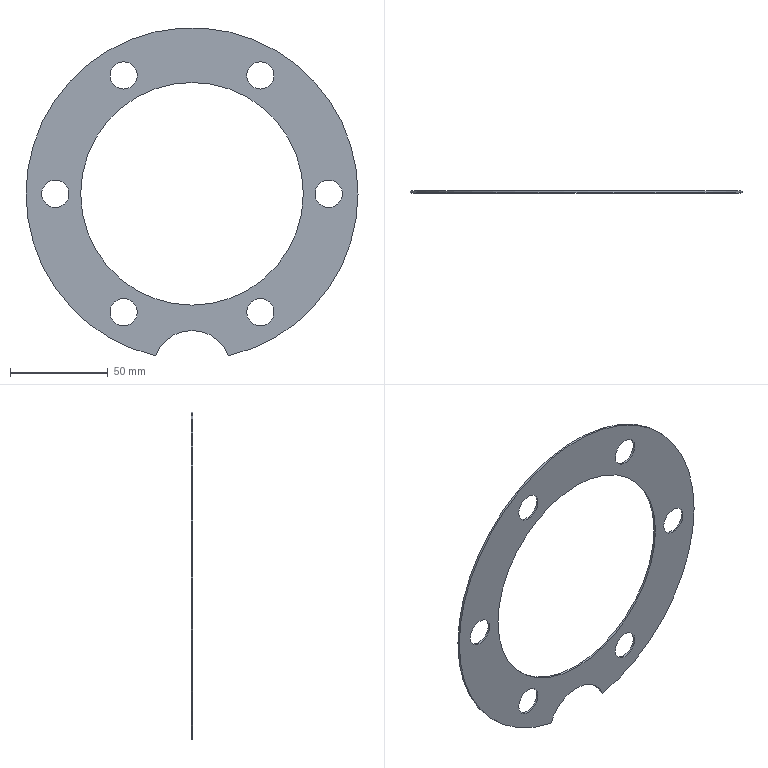Part | SolidWorks | features Extrusion 1 | 1 solid | 18 faces | box 170 x 1 x 167.917 mm | volume 11164 mm3 | cylinder 16 | plane 2 | commonest cylinder face diameters 14 x12 114 x2 40 x1 170 x1
STEP:
#1=CARTESIAN_POINT('',(-70.,1.,-7.));
#2=VERTEX_POINT('',#1);
#3=CARTESIAN_POINT('',(-70.,1.,7.));
#4=VERTEX_POINT('',#3);
#5=CARTESIAN_POINT('',(-70.,1.,0.));
#6=DIRECTION('',(0.,1.,0.));
#7=DIRECTION('',(0.,0.,1.));
#8=AXIS2_PLACEMENT_3D('',#5,#6,#7);
#9=CIRCLE('',#8,7.);
#10=EDGE_CURVE('',#2,#4,#9,.T.);
#11=ORIENTED_EDGE('',*,*,#10,.T.);
#12=CARTESIAN_POINT('',(-70.,0.,7.));
#13=VERTEX_POINT('',#12);
#14=CARTESIAN_POINT('',(-70.,1.,7.));
#15=DIRECTION('',(0.,-1.,0.));
#16=VECTOR('',#15,1000.);
#17=LINE('',#14,#16);
#18=EDGE_CURVE('',#4,#13,#17,.T.);
#19=ORIENTED_EDGE('',*,*,#18,.T.);
#20=CARTESIAN_POINT('',(-70.,0.,-7.));
#21=VERTEX_POINT('',#20);
#22=CARTESIAN_POINT('',(-70.,0.,0.));
#23=DIRECTION('',(0.,1.,0.));
#24=DIRECTION('',(0.,0.,1.));
#25=AXIS2_PLACEMENT_3D('',#22,#23,#24);
#26=CIRCLE('',#25,7.);
#27=EDGE_CURVE('',#21,#13,#26,.T.);
#28=ORIENTED_EDGE('',*,*,#27,.F.);
#29=CARTESIAN_POINT('',(-70.,1.,-7.));
#30=DIRECTION('',(0.,-1.,0.));
#31=VECTOR('',#30,1000.);
#32=LINE('',#29,#31);
#33=EDGE_CURVE('',#2,#21,#32,.T.);
#34=ORIENTED_EDGE('',*,*,#33,.F.);
#35=EDGE_LOOP('',(#11,#19,#28,#34));
#36=FACE_OUTER_BOUND('',#35,.T.);
#37=CARTESIAN_POINT('',(-70.,1.,0.));
#38=DIRECTION('',(0.,-1.,0.));
#39=DIRECTION('',(0.,0.,-1.));
#40=AXIS2_PLACEMENT_3D('',#37,#38,#39);
#41=CYLINDRICAL_SURFACE('',#40,7.);
#42=ADVANCED_FACE('',(#36),#41,.F.);
#43=CARTESIAN_POINT('',(-35.,1.,53.622));
#44=VERTEX_POINT('',#43);
#45=CARTESIAN_POINT('',(-35.,1.,67.622));
#46=VERTEX_POINT('',#45);
#47=CARTESIAN_POINT('',(-35.,1.,60.622));
#48=DIRECTION('',(0.,1.,0.));
#49=DIRECTION('',(0.,0.,1.));
#50=AXIS2_PLACEMENT_3D('',#47,#48,#49);
#51=CIRCLE('',#50,7.);
#52=EDGE_CURVE('',#44,#46,#51,.T.);
#53=ORIENTED_EDGE('',*,*,#52,.T.);
#54=CARTESIAN_POINT('',(-35.,0.,67.622));
#55=VERTEX_POINT('',#54);
#56=CARTESIAN_POINT('',(-35.,1.,67.622));
#57=DIRECTION('',(0.,-1.,0.));
#58=VECTOR('',#57,1000.);
#59=LINE('',#56,#58);
#60=EDGE_CURVE('',#46,#55,#59,.T.);
#61=ORIENTED_EDGE('',*,*,#60,.T.);
#62=CARTESIAN_POINT('',(-35.,0.,53.622));
#63=VERTEX_POINT('',#62);
#64=CARTESIAN_POINT('',(-35.,0.,60.622));
#65=DIRECTION('',(0.,1.,0.));
#66=DIRECTION('',(0.,0.,1.));
#67=AXIS2_PLACEMENT_3D('',#64,#65,#66);
#68=CIRCLE('',#67,7.);
#69=EDGE_CURVE('',#63,#55,#68,.T.);
#70=ORIENTED_EDGE('',*,*,#69,.F.);
#71=CARTESIAN_POINT('',(-35.,1.,53.622));
#72=DIRECTION('',(0.,-1.,0.));
#73=VECTOR('',#72,1000.);
#74=LINE('',#71,#73);
#75=EDGE_CURVE('',#44,#63,#74,.T.);
#76=ORIENTED_EDGE('',*,*,#75,.F.);
#77=EDGE_LOOP('',(#53,#61,#70,#76));
#78=FACE_OUTER_BOUND('',#77,.T.);
#79=CARTESIAN_POINT('',(-35.,1.,60.622));
#80=DIRECTION('',(0.,-1.,0.));
#81=DIRECTION('',(0.,0.,-1.));
#82=AXIS2_PLACEMENT_3D('',#79,#80,#81);
#83=CYLINDRICAL_SURFACE('',#82,7.);
#84=ADVANCED_FACE('',(#78),#83,.F.);
#85=CARTESIAN_POINT('',(35.,1.,53.622));
#86=VERTEX_POINT('',#85);
#87=CARTESIAN_POINT('',(35.,1.,67.622));
#88=VERTEX_POINT('',#87);
#89=CARTESIAN_POINT('',(35.,1.,60.622));
#90=DIRECTION('',(0.,1.,0.));
#91=DIRECTION('',(0.,0.,1.));
#92=AXIS2_PLACEMENT_3D('',#89,#90,#91);
#93=CIRCLE('',#92,7.);
#94=EDGE_CURVE('',#86,#88,#93,.T.);
#95=ORIENTED_EDGE('',*,*,#94,.T.);
#96=CARTESIAN_POINT('',(35.,0.,67.622));
#97=VERTEX_POINT('',#96);
#98=CARTESIAN_POINT('',(35.,1.,67.622));
#99=DIRECTION('',(0.,-1.,0.));
#100=VECTOR('',#99,1000.);
#101=LINE('',#98,#100);
#102=EDGE_CURVE('',#88,#97,#101,.T.);
#103=ORIENTED_EDGE('',*,*,#102,.T.);
#104=CARTESIAN_POINT('',(35.,0.,53.622));
#105=VERTEX_POINT('',#104);
#106=CARTESIAN_POINT('',(35.,0.,60.622));
#107=DIRECTION('',(0.,1.,0.));
#108=DIRECTION('',(0.,0.,1.));
#109=AXIS2_PLACEMENT_3D('',#106,#107,#108);
#110=CIRCLE('',#109,7.);
#111=EDGE_CURVE('',#105,#97,#110,.T.);
#112=ORIENTED_EDGE('',*,*,#111,.F.);
#113=CARTESIAN_POINT('',(35.,1.,53.622));
#114=DIRECTION('',(0.,-1.,0.));
#115=VECTOR('',#114,1000.);
#116=LINE('',#113,#115);
#117=EDGE_CURVE('',#86,#105,#116,.T.);
#118=ORIENTED_EDGE('',*,*,#117,.F.);
#119=EDGE_LOOP('',(#95,#103,#112,#118));
#120=FACE_OUTER_BOUND('',#119,.T.);
#121=CARTESIAN_POINT('',(35.,1.,60.622));
#122=DIRECTION('',(0.,-1.,0.));
#123=DIRECTION('',(0.,0.,-1.));
#124=AXIS2_PLACEMENT_3D('',#121,#122,#123);
#125=CYLINDRICAL_SURFACE('',#124,7.);
#126=ADVANCED_FACE('',(#120),#125,.F.);
#127=CARTESIAN_POINT('',(70.,1.,-7.));
#128=VERTEX_POINT('',#127);
#129=CARTESIAN_POINT('',(70.,1.,7.));
#130=VERTEX_POINT('',#129);
#131=CARTESIAN_POINT('',(70.,1.,0.));
#132=DIRECTION('',(0.,1.,0.));
#133=DIRECTION('',(0.,0.,1.));
#134=AXIS2_PLACEMENT_3D('',#131,#132,#133);
#135=CIRCLE('',#134,7.);
#136=EDGE_CURVE('',#128,#130,#135,.T.);
#137=ORIENTED_EDGE('',*,*,#136,.T.);
#138=CARTESIAN_POINT('',(70.,0.,7.));
#139=VERTEX_POINT('',#138);
#140=CARTESIAN_POINT('',(70.,1.,7.));
#141=DIRECTION('',(0.,-1.,0.));
#142=VECTOR('',#141,1000.);
#143=LINE('',#140,#142);
#144=EDGE_CURVE('',#130,#139,#143,.T.);
#145=ORIENTED_EDGE('',*,*,#144,.T.);
#146=CARTESIAN_POINT('',(70.,0.,-7.));
#147=VERTEX_POINT('',#146);
#148=CARTESIAN_POINT('',(70.,0.,0.));
#149=DIRECTION('',(0.,1.,0.));
#150=DIRECTION('',(0.,0.,1.));
#151=AXIS2_PLACEMENT_3D('',#148,#149,#150);
#152=CIRCLE('',#151,7.);
#153=EDGE_CURVE('',#147,#139,#152,.T.);
#154=ORIENTED_EDGE('',*,*,#153,.F.);
#155=CARTESIAN_POINT('',(70.,1.,-7.));
#156=DIRECTION('',(0.,-1.,0.));
#157=VECTOR('',#156,1000.);
#158=LINE('',#155,#157);
#159=EDGE_CURVE('',#128,#147,#158,.T.);
#160=ORIENTED_EDGE('',*,*,#159,.F.);
#161=EDGE_LOOP('',(#137,#145,#154,#160));
#162=FACE_OUTER_BOUND('',#161,.T.);
#163=CARTESIAN_POINT('',(70.,1.,0.));
#164=DIRECTION('',(0.,-1.,0.));
#165=DIRECTION('',(0.,0.,-1.));
#166=AXIS2_PLACEMENT_3D('',#163,#164,#165);
#167=CYLINDRICAL_SURFACE('',#166,7.);
#168=ADVANCED_FACE('',(#162),#167,.F.);
#169=CARTESIAN_POINT('',(35.,1.,-67.622));
#170=VERTEX_POINT('',#169);
#171=CARTESIAN_POINT('',(35.,1.,-53.622));
#172=VERTEX_POINT('',#171);
#173=CARTESIAN_POINT('',(35.,1.,-60.622));
#174=DIRECTION('',(0.,1.,0.));
#175=DIRECTION('',(0.,0.,1.));
#176=AXIS2_PLACEMENT_3D('',#173,#174,#175);
#177=CIRCLE('',#176,7.);
#178=EDGE_CURVE('',#170,#172,#177,.T.);
#179=ORIENTED_EDGE('',*,*,#178,.T.);
#180=CARTESIAN_POINT('',(35.,0.,-53.622));
#181=VERTEX_POINT('',#180);
#182=CARTESIAN_POINT('',(35.,1.,-53.622));
#183=DIRECTION('',(0.,-1.,0.));
#184=VECTOR('',#183,1000.);
#185=LINE('',#182,#184);
#186=EDGE_CURVE('',#172,#181,#185,.T.);
#187=ORIENTED_EDGE('',*,*,#186,.T.);
#188=CARTESIAN_POINT('',(35.,0.,-67.622));
#189=VERTEX_POINT('',#188);
#190=CARTESIAN_POINT('',(35.,0.,-60.622));
#191=DIRECTION('',(0.,1.,0.));
#192=DIRECTION('',(0.,0.,1.));
#193=AXIS2_PLACEMENT_3D('',#190,#191,#192);
#194=CIRCLE('',#193,7.);
#195=EDGE_CURVE('',#189,#181,#194,.T.);
#196=ORIENTED_EDGE('',*,*,#195,.F.);
#197=CARTESIAN_POINT('',(35.,1.,-67.622));
#198=DIRECTION('',(0.,-1.,0.));
#199=VECTOR('',#198,1000.);
#200=LINE('',#197,#199);
#201=EDGE_CURVE('',#170,#189,#200,.T.);
#202=ORIENTED_EDGE('',*,*,#201,.F.);
#203=EDGE_LOOP('',(#179,#187,#196,#202));
#204=FACE_OUTER_BOUND('',#203,.T.);
#205=CARTESIAN_POINT('',(35.,1.,-60.622));
#206=DIRECTION('',(0.,-1.,0.));
#207=DIRECTION('',(0.,0.,-1.));
#208=AXIS2_PLACEMENT_3D('',#205,#206,#207);
#209=CYLINDRICAL_SURFACE('',#208,7.);
#210=ADVANCED_FACE('',(#204),#209,.F.);
#211=CARTESIAN_POINT('',(-35.,1.,-67.622));
#212=VERTEX_POINT('',#211);
#213=CARTESIAN_POINT('',(-35.,1.,-53.622));
#214=VERTEX_POINT('',#213);
#215=CARTESIAN_POINT('',(-35.,1.,-60.622));
#216=DIRECTION('',(0.,1.,0.));
#217=DIRECTION('',(0.,0.,1.));
#218=AXIS2_PLACEMENT_3D('',#215,#216,#217);
#219=CIRCLE('',#218,7.);
#220=EDGE_CURVE('',#212,#214,#219,.T.);
#221=ORIENTED_EDGE('',*,*,#220,.T.);
#222=CARTESIAN_POINT('',(-35.,0.,-53.622));
#223=VERTEX_POINT('',#222);
#224=CARTESIAN_POINT('',(-35.,1.,-53.622));
#225=DIRECTION('',(0.,-1.,0.));
#226=VECTOR('',#225,1000.);
#227=LINE('',#224,#226);
#228=EDGE_CURVE('',#214,#223,#227,.T.);
#229=ORIENTED_EDGE('',*,*,#228,.T.);
#230=CARTESIAN_POINT('',(-35.,0.,-67.622));
#231=VERTEX_POINT('',#230);
#232=CARTESIAN_POINT('',(-35.,0.,-60.622));
#233=DIRECTION('',(0.,1.,0.));
#234=DIRECTION('',(0.,0.,1.));
#235=AXIS2_PLACEMENT_3D('',#232,#233,#234);
#236=CIRCLE('',#235,7.);
#237=EDGE_CURVE('',#231,#223,#236,.T.);
#238=ORIENTED_EDGE('',*,*,#237,.F.);
#239=CARTESIAN_POINT('',(-35.,1.,-67.622));
#240=DIRECTION('',(0.,-1.,0.));
#241=VECTOR('',#240,1000.);
#242=LINE('',#239,#241);
#243=EDGE_CURVE('',#212,#231,#242,.T.);
#244=ORIENTED_EDGE('',*,*,#243,.F.);
#245=EDGE_LOOP('',(#221,#229,#238,#244));
#246=FACE_OUTER_BOUND('',#245,.T.);
#247=CARTESIAN_POINT('',(-35.,1.,-60.622));
#248=DIRECTION('',(0.,-1.,0.));
#249=DIRECTION('',(0.,0.,-1.));
#250=AXIS2_PLACEMENT_3D('',#247,#248,#249);
#251=CYLINDRICAL_SURFACE('',#250,7.);
#252=ADVANCED_FACE('',(#246),#251,.F.);
#253=CARTESIAN_POINT('',(0.,1.,-57.));
#254=VERTEX_POINT('',#253);
#255=CARTESIAN_POINT('',(0.,1.,57.));
#256=VERTEX_POINT('',#255);
#257=CARTESIAN_POINT('',(0.,1.,0.));
#258=DIRECTION('',(0.,1.,0.));
#259=DIRECTION('',(0.,0.,1.));
#260=AXIS2_PLACEMENT_3D('',#257,#258,#259);
#261=CIRCLE('',#260,57.);
#262=EDGE_CURVE('',#254,#256,#261,.T.);
#263=ORIENTED_EDGE('',*,*,#262,.T.);
#264=CARTESIAN_POINT('',(0.,0.,57.));
#265=VERTEX_POINT('',#264);
#266=CARTESIAN_POINT('',(0.,1.,57.));
#267=DIRECTION('',(0.,-1.,0.));
#268=VECTOR('',#267,1000.);
#269=LINE('',#266,#268);
#270=EDGE_CURVE('',#256,#265,#269,.T.);
#271=ORIENTED_EDGE('',*,*,#270,.T.);
#272=CARTESIAN_POINT('',(0.,0.,-57.));
#273=VERTEX_POINT('',#272);
#274=CARTESIAN_POINT('',(0.,0.,0.));
#275=DIRECTION('',(0.,1.,0.));
#276=DIRECTION('',(0.,0.,1.));
#277=AXIS2_PLACEMENT_3D('',#274,#275,#276);
#278=CIRCLE('',#277,57.);
#279=EDGE_CURVE('',#273,#265,#278,.T.);
#280=ORIENTED_EDGE('',*,*,#279,.F.);
#281=CARTESIAN_POINT('',(0.,1.,-57.));
#282=DIRECTION('',(0.,-1.,0.));
#283=VECTOR('',#282,1000.);
#284=LINE('',#281,#283);
#285=EDGE_CURVE('',#254,#273,#284,.T.);
#286=ORIENTED_EDGE('',*,*,#285,.F.);
#287=EDGE_LOOP('',(#263,#271,#280,#286));
#288=FACE_OUTER_BOUND('',#287,.T.);
#289=CARTESIAN_POINT('',(0.,1.,0.));
#290=DIRECTION('',(0.,-1.,0.));
#291=DIRECTION('',(0.,0.,-1.));
#292=AXIS2_PLACEMENT_3D('',#289,#290,#291);
#293=CYLINDRICAL_SURFACE('',#292,57.);
#294=ADVANCED_FACE('',(#288),#293,.F.);
#295=ORIENTED_EDGE('',*,*,#52,.F.);
#296=CARTESIAN_POINT('',(-35.,1.,60.622));
#297=DIRECTION('',(0.,1.,0.));
#298=DIRECTION('',(0.,0.,1.));
#299=AXIS2_PLACEMENT_3D('',#296,#297,#298);
#300=CIRCLE('',#299,7.);
#301=EDGE_CURVE('',#46,#44,#300,.T.);
#302=ORIENTED_EDGE('',*,*,#301,.F.);
#303=EDGE_LOOP('',(#295,#302));
#304=FACE_BOUND('',#303,.T.);
#305=ORIENTED_EDGE('',*,*,#136,.F.);
#306=CARTESIAN_POINT('',(70.,1.,0.));
#307=DIRECTION('',(0.,1.,0.));
#308=DIRECTION('',(0.,0.,1.));
#309=AXIS2_PLACEMENT_3D('',#306,#307,#308);
#310=CIRCLE('',#309,7.);
#311=EDGE_CURVE('',#130,#128,#310,.T.);
#312=ORIENTED_EDGE('',*,*,#311,.F.);
#313=EDGE_LOOP('',(#305,#312));
#314=FACE_BOUND('',#313,.T.);
#315=ORIENTED_EDGE('',*,*,#220,.F.);
#316=CARTESIAN_POINT('',(-35.,1.,-60.622));
#317=DIRECTION('',(0.,1.,0.));
#318=DIRECTION('',(0.,0.,1.));
#319=AXIS2_PLACEMENT_3D('',#316,#317,#318);
#320=CIRCLE('',#319,7.);
#321=EDGE_CURVE('',#214,#212,#320,.T.);
#322=ORIENTED_EDGE('',*,*,#321,.F.);
#323=EDGE_LOOP('',(#315,#322));
#324=FACE_BOUND('',#323,.T.);
#325=CARTESIAN_POINT('',(18.704,1.,-82.917));
#326=VERTEX_POINT('',#325);
#327=CARTESIAN_POINT('',(-18.704,1.,-82.917));
#328=VERTEX_POINT('',#327);
#329=CARTESIAN_POINT('',(0.,1.,-90.));
#330=DIRECTION('',(0.,-1.,0.));
#331=DIRECTION('',(0.,0.,1.));
#332=AXIS2_PLACEMENT_3D('',#329,#330,#331);
#333=CIRCLE('',#332,20.);
#334=EDGE_CURVE('',#326,#328,#333,.T.);
#335=ORIENTED_EDGE('',*,*,#334,.T.);
#336=CARTESIAN_POINT('',(0.,1.,0.));
#337=DIRECTION('',(0.,1.,0.));
#338=DIRECTION('',(0.,0.,1.));
#339=AXIS2_PLACEMENT_3D('',#336,#337,#338);
#340=CIRCLE('',#339,85.);
#341=EDGE_CURVE('',#328,#326,#340,.T.);
#342=ORIENTED_EDGE('',*,*,#341,.T.);
#343=EDGE_LOOP('',(#335,#342));
#344=FACE_OUTER_BOUND('',#343,.T.);
#345=ORIENTED_EDGE('',*,*,#262,.F.);
#346=CARTESIAN_POINT('',(0.,1.,0.));
#347=DIRECTION('',(0.,1.,0.));
#348=DIRECTION('',(0.,0.,1.));
#349=AXIS2_PLACEMENT_3D('',#346,#347,#348);
#350=CIRCLE('',#349,57.);
#351=EDGE_CURVE('',#256,#254,#350,.T.);
#352=ORIENTED_EDGE('',*,*,#351,.F.);
#353=EDGE_LOOP('',(#345,#352));
#354=FACE_BOUND('',#353,.T.);
#355=ORIENTED_EDGE('',*,*,#178,.F.);
#356=CARTESIAN_POINT('',(35.,1.,-60.622));
#357=DIRECTION('',(0.,1.,0.));
#358=DIRECTION('',(0.,0.,1.));
#359=AXIS2_PLACEMENT_3D('',#356,#357,#358);
#360=CIRCLE('',#359,7.);
#361=EDGE_CURVE('',#172,#170,#360,.T.);
#362=ORIENTED_EDGE('',*,*,#361,.F.);
#363=EDGE_LOOP('',(#355,#362));
#364=FACE_BOUND('',#363,.T.);
#365=ORIENTED_EDGE('',*,*,#94,.F.);
#366=CARTESIAN_POINT('',(35.,1.,60.622));
#367=DIRECTION('',(0.,1.,0.));
#368=DIRECTION('',(0.,0.,1.));
#369=AXIS2_PLACEMENT_3D('',#366,#367,#368);
#370=CIRCLE('',#369,7.);
#371=EDGE_CURVE('',#88,#86,#370,.T.);
#372=ORIENTED_EDGE('',*,*,#371,.F.);
#373=EDGE_LOOP('',(#365,#372));
#374=FACE_BOUND('',#373,.T.);
#375=ORIENTED_EDGE('',*,*,#10,.F.);
#376=CARTESIAN_POINT('',(-70.,1.,0.));
#377=DIRECTION('',(0.,1.,0.));
#378=DIRECTION('',(0.,0.,1.));
#379=AXIS2_PLACEMENT_3D('',#376,#377,#378);
#380=CIRCLE('',#379,7.);
#381=EDGE_CURVE('',#4,#2,#380,.T.);
#382=ORIENTED_EDGE('',*,*,#381,.F.);
#383=EDGE_LOOP('',(#375,#382));
#384=FACE_BOUND('',#383,.T.);
#385=CARTESIAN_POINT('',(0.,1.,-45.));
#386=DIRECTION('',(0.,1.,0.));
#387=DIRECTION('',(0.,0.,1.));
#388=AXIS2_PLACEMENT_3D('',#385,#386,#387);
#389=PLANE('',#388);
#390=ADVANCED_FACE('',(#304,#314,#324,#344,#354,#364,#374,#384),#389,.T.);
#391=CARTESIAN_POINT('',(18.704,0.,-82.917));
#392=VERTEX_POINT('',#391);
#393=CARTESIAN_POINT('',(-18.704,0.,-82.917));
#394=VERTEX_POINT('',#393);
#395=CARTESIAN_POINT('',(0.,0.,-90.));
#396=DIRECTION('',(0.,-1.,0.));
#397=DIRECTION('',(0.,0.,1.));
#398=AXIS2_PLACEMENT_3D('',#395,#396,#397);
#399=CIRCLE('',#398,20.);
#400=EDGE_CURVE('',#392,#394,#399,.T.);
#401=ORIENTED_EDGE('',*,*,#400,.F.);
#402=CARTESIAN_POINT('',(0.,0.,0.));
#403=DIRECTION('',(0.,1.,0.));
#404=DIRECTION('',(0.,0.,1.));
#405=AXIS2_PLACEMENT_3D('',#402,#403,#404);
#406=CIRCLE('',#405,85.);
#407=EDGE_CURVE('',#394,#392,#406,.T.);
#408=ORIENTED_EDGE('',*,*,#407,.F.);
#409=EDGE_LOOP('',(#401,#408));
#410=FACE_OUTER_BOUND('',#409,.T.);
#411=ORIENTED_EDGE('',*,*,#279,.T.);
#412=CARTESIAN_POINT('',(0.,0.,0.));
#413=DIRECTION('',(0.,1.,0.));
#414=DIRECTION('',(0.,0.,1.));
#415=AXIS2_PLACEMENT_3D('',#412,#413,#414);
#416=CIRCLE('',#415,57.);
#417=EDGE_CURVE('',#265,#273,#416,.T.);
#418=ORIENTED_EDGE('',*,*,#417,.T.);
#419=EDGE_LOOP('',(#411,#418));
#420=FACE_BOUND('',#419,.T.);
#421=ORIENTED_EDGE('',*,*,#237,.T.);
#422=CARTESIAN_POINT('',(-35.,0.,-60.622));
#423=DIRECTION('',(0.,1.,0.));
#424=DIRECTION('',(0.,0.,1.));
#425=AXIS2_PLACEMENT_3D('',#422,#423,#424);
#426=CIRCLE('',#425,7.);
#427=EDGE_CURVE('',#223,#231,#426,.T.);
#428=ORIENTED_EDGE('',*,*,#427,.T.);
#429=EDGE_LOOP('',(#421,#428));
#430=FACE_BOUND('',#429,.T.);
#431=ORIENTED_EDGE('',*,*,#195,.T.);
#432=CARTESIAN_POINT('',(35.,0.,-60.622));
#433=DIRECTION('',(0.,1.,0.));
#434=DIRECTION('',(0.,0.,1.));
#435=AXIS2_PLACEMENT_3D('',#432,#433,#434);
#436=CIRCLE('',#435,7.);
#437=EDGE_CURVE('',#181,#189,#436,.T.);
#438=ORIENTED_EDGE('',*,*,#437,.T.);
#439=EDGE_LOOP('',(#431,#438));
#440=FACE_BOUND('',#439,.T.);
#441=ORIENTED_EDGE('',*,*,#153,.T.);
#442=CARTESIAN_POINT('',(70.,0.,0.));
#443=DIRECTION('',(0.,1.,0.));
#444=DIRECTION('',(0.,0.,1.));
#445=AXIS2_PLACEMENT_3D('',#442,#443,#444);
#446=CIRCLE('',#445,7.);
#447=EDGE_CURVE('',#139,#147,#446,.T.);
#448=ORIENTED_EDGE('',*,*,#447,.T.);
#449=EDGE_LOOP('',(#441,#448));
#450=FACE_BOUND('',#449,.T.);
#451=ORIENTED_EDGE('',*,*,#111,.T.);
#452=CARTESIAN_POINT('',(35.,0.,60.622));
#453=DIRECTION('',(0.,1.,0.));
#454=DIRECTION('',(0.,0.,1.));
#455=AXIS2_PLACEMENT_3D('',#452,#453,#454);
#456=CIRCLE('',#455,7.);
#457=EDGE_CURVE('',#97,#105,#456,.T.);
#458=ORIENTED_EDGE('',*,*,#457,.T.);
#459=EDGE_LOOP('',(#451,#458));
#460=FACE_BOUND('',#459,.T.);
#461=ORIENTED_EDGE('',*,*,#69,.T.);
#462=CARTESIAN_POINT('',(-35.,0.,60.622));
#463=DIRECTION('',(0.,1.,0.));
#464=DIRECTION('',(0.,0.,1.));
#465=AXIS2_PLACEMENT_3D('',#462,#463,#464);
#466=CIRCLE('',#465,7.);
#467=EDGE_CURVE('',#55,#63,#466,.T.);
#468=ORIENTED_EDGE('',*,*,#467,.T.);
#469=EDGE_LOOP('',(#461,#468));
#470=FACE_BOUND('',#469,.T.);
#471=ORIENTED_EDGE('',*,*,#27,.T.);
#472=CARTESIAN_POINT('',(-70.,0.,0.));
#473=DIRECTION('',(0.,1.,0.));
#474=DIRECTION('',(0.,0.,1.));
#475=AXIS2_PLACEMENT_3D('',#472,#473,#474);
#476=CIRCLE('',#475,7.);
#477=EDGE_CURVE('',#13,#21,#476,.T.);
#478=ORIENTED_EDGE('',*,*,#477,.T.);
#479=EDGE_LOOP('',(#471,#478));
#480=FACE_BOUND('',#479,.T.);
#481=CARTESIAN_POINT('',(0.,0.,-45.));
#482=DIRECTION('',(0.,1.,0.));
#483=DIRECTION('',(0.,0.,1.));
#484=AXIS2_PLACEMENT_3D('',#481,#482,#483);
#485=PLANE('',#484);
#486=ADVANCED_FACE('',(#410,#420,#430,#440,#450,#460,#470,#480),#485,.F.);
#487=ORIENTED_EDGE('',*,*,#400,.T.);
#488=CARTESIAN_POINT('',(-18.704,1.,-82.917));
#489=DIRECTION('',(0.,-1.,0.));
#490=VECTOR('',#489,1000.);
#491=LINE('',#488,#490);
#492=EDGE_CURVE('',#328,#394,#491,.T.);
#493=ORIENTED_EDGE('',*,*,#492,.F.);
#494=ORIENTED_EDGE('',*,*,#334,.F.);
#495=CARTESIAN_POINT('',(18.704,1.,-82.917));
#496=DIRECTION('',(0.,-1.,0.));
#497=VECTOR('',#496,1000.);
#498=LINE('',#495,#497);
#499=EDGE_CURVE('',#326,#392,#498,.T.);
#500=ORIENTED_EDGE('',*,*,#499,.T.);
#501=EDGE_LOOP('',(#487,#493,#494,#500));
#502=FACE_OUTER_BOUND('',#501,.T.);
#503=CARTESIAN_POINT('',(0.,1.,-90.));
#504=DIRECTION('',(0.,-1.,0.));
#505=DIRECTION('',(0.,0.,-1.));
#506=AXIS2_PLACEMENT_3D('',#503,#504,#505);
#507=CYLINDRICAL_SURFACE('',#506,20.);
#508=ADVANCED_FACE('',(#502),#507,.F.);
#509=ORIENTED_EDGE('',*,*,#407,.T.);
#510=ORIENTED_EDGE('',*,*,#499,.F.);
#511=ORIENTED_EDGE('',*,*,#341,.F.);
#512=ORIENTED_EDGE('',*,*,#492,.T.);
#513=EDGE_LOOP('',(#509,#510,#511,#512));
#514=FACE_OUTER_BOUND('',#513,.T.);
#515=CARTESIAN_POINT('',(0.,1.,0.));
#516=DIRECTION('',(0.,-1.,0.));
#517=DIRECTION('',(0.,0.,-1.));
#518=AXIS2_PLACEMENT_3D('',#515,#516,#517);
#519=CYLINDRICAL_SURFACE('',#518,85.);
#520=ADVANCED_FACE('',(#514),#519,.T.);
#521=ORIENTED_EDGE('',*,*,#270,.F.);
#522=ORIENTED_EDGE('',*,*,#351,.T.);
#523=ORIENTED_EDGE('',*,*,#285,.T.);
#524=ORIENTED_EDGE('',*,*,#417,.F.);
#525=EDGE_LOOP('',(#521,#522,#523,#524));
#526=FACE_OUTER_BOUND('',#525,.T.);
#527=CARTESIAN_POINT('',(0.,1.,0.));
#528=DIRECTION('',(0.,-1.,0.));
#529=DIRECTION('',(0.,0.,-1.));
#530=AXIS2_PLACEMENT_3D('',#527,#528,#529);
#531=CYLINDRICAL_SURFACE('',#530,57.);
#532=ADVANCED_FACE('',(#526),#531,.F.);
#533=ORIENTED_EDGE('',*,*,#228,.F.);
#534=ORIENTED_EDGE('',*,*,#321,.T.);
#535=ORIENTED_EDGE('',*,*,#243,.T.);
#536=ORIENTED_EDGE('',*,*,#427,.F.);
#537=EDGE_LOOP('',(#533,#534,#535,#536));
#538=FACE_OUTER_BOUND('',#537,.T.);
#539=CARTESIAN_POINT('',(-35.,1.,-60.622));
#540=DIRECTION('',(0.,-1.,0.));
#541=DIRECTION('',(0.,0.,-1.));
#542=AXIS2_PLACEMENT_3D('',#539,#540,#541);
#543=CYLINDRICAL_SURFACE('',#542,7.);
#544=ADVANCED_FACE('',(#538),#543,.F.);
#545=ORIENTED_EDGE('',*,*,#186,.F.);
#546=ORIENTED_EDGE('',*,*,#361,.T.);
#547=ORIENTED_EDGE('',*,*,#201,.T.);
#548=ORIENTED_EDGE('',*,*,#437,.F.);
#549=EDGE_LOOP('',(#545,#546,#547,#548));
#550=FACE_OUTER_BOUND('',#549,.T.);
#551=CARTESIAN_POINT('',(35.,1.,-60.622));
#552=DIRECTION('',(0.,-1.,0.));
#553=DIRECTION('',(0.,0.,-1.));
#554=AXIS2_PLACEMENT_3D('',#551,#552,#553);
#555=CYLINDRICAL_SURFACE('',#554,7.);
#556=ADVANCED_FACE('',(#550),#555,.F.);
#557=ORIENTED_EDGE('',*,*,#144,.F.);
#558=ORIENTED_EDGE('',*,*,#311,.T.);
#559=ORIENTED_EDGE('',*,*,#159,.T.);
#560=ORIENTED_EDGE('',*,*,#447,.F.);
#561=EDGE_LOOP('',(#557,#558,#559,#560));
#562=FACE_OUTER_BOUND('',#561,.T.);
#563=CARTESIAN_POINT('',(70.,1.,0.));
#564=DIRECTION('',(0.,-1.,0.));
#565=DIRECTION('',(0.,0.,-1.));
#566=AXIS2_PLACEMENT_3D('',#563,#564,#565);
#567=CYLINDRICAL_SURFACE('',#566,7.);
#568=ADVANCED_FACE('',(#562),#567,.F.);
#569=ORIENTED_EDGE('',*,*,#102,.F.);
#570=ORIENTED_EDGE('',*,*,#371,.T.);
#571=ORIENTED_EDGE('',*,*,#117,.T.);
#572=ORIENTED_EDGE('',*,*,#457,.F.);
#573=EDGE_LOOP('',(#569,#570,#571,#572));
#574=FACE_OUTER_BOUND('',#573,.T.);
#575=CARTESIAN_POINT('',(35.,1.,60.622));
#576=DIRECTION('',(0.,-1.,0.));
#577=DIRECTION('',(0.,0.,-1.));
#578=AXIS2_PLACEMENT_3D('',#575,#576,#577);
#579=CYLINDRICAL_SURFACE('',#578,7.);
#580=ADVANCED_FACE('',(#574),#579,.F.);
#581=ORIENTED_EDGE('',*,*,#60,.F.);
#582=ORIENTED_EDGE('',*,*,#301,.T.);
#583=ORIENTED_EDGE('',*,*,#75,.T.);
#584=ORIENTED_EDGE('',*,*,#467,.F.);
#585=EDGE_LOOP('',(#581,#582,#583,#584));
#586=FACE_OUTER_BOUND('',#585,.T.);
#587=CARTESIAN_POINT('',(-35.,1.,60.622));
#588=DIRECTION('',(0.,-1.,0.));
#589=DIRECTION('',(0.,0.,-1.));
#590=AXIS2_PLACEMENT_3D('',#587,#588,#589);
#591=CYLINDRICAL_SURFACE('',#590,7.);
#592=ADVANCED_FACE('',(#586),#591,.F.);
#593=ORIENTED_EDGE('',*,*,#18,.F.);
#594=ORIENTED_EDGE('',*,*,#381,.T.);
#595=ORIENTED_EDGE('',*,*,#33,.T.);
#596=ORIENTED_EDGE('',*,*,#477,.F.);
#597=EDGE_LOOP('',(#593,#594,#595,#596));
#598=FACE_OUTER_BOUND('',#597,.T.);
#599=CARTESIAN_POINT('',(-70.,1.,0.));
#600=DIRECTION('',(0.,-1.,0.));
#601=DIRECTION('',(0.,0.,-1.));
#602=AXIS2_PLACEMENT_3D('',#599,#600,#601);
#603=CYLINDRICAL_SURFACE('',#602,7.);
#604=ADVANCED_FACE('',(#598),#603,.F.);
#605=CLOSED_SHELL('',(#42,#84,#126,#168,#210,#252,#294,#390,#486,#508,#520,#532,#544,#556,#568,#580,#592,#604));
#606=MANIFOLD_SOLID_BREP('',#605);
#607=CARTESIAN_POINT('',(0.,0.,0.));
#608=DIRECTION('',(0.,0.,1.));
#609=DIRECTION('',(1.,0.,0.));
#610=AXIS2_PLACEMENT_3D('',#607,#608,#609);
#611=(LENGTH_UNIT()NAMED_UNIT(*)SI_UNIT(.MILLI.,.METRE.));
#612=UNCERTAINTY_MEASURE_WITH_UNIT(LENGTH_MEASURE(0.00001),#611,'','');
#613=(NAMED_UNIT(*)PLANE_ANGLE_UNIT()SI_UNIT($,.RADIAN.));
#614=(NAMED_UNIT(*)SI_UNIT($,.STERADIAN.)SOLID_ANGLE_UNIT());
#615=(GEOMETRIC_REPRESENTATION_CONTEXT(3)GLOBAL_UNCERTAINTY_ASSIGNED_CONTEXT((#612))GLOBAL_UNIT_ASSIGNED_CONTEXT((#611,#613,#614))REPRESENTATION_CONTEXT('',''));
#616=ADVANCED_BREP_SHAPE_REPRESENTATION('',(#606,#610),#615);